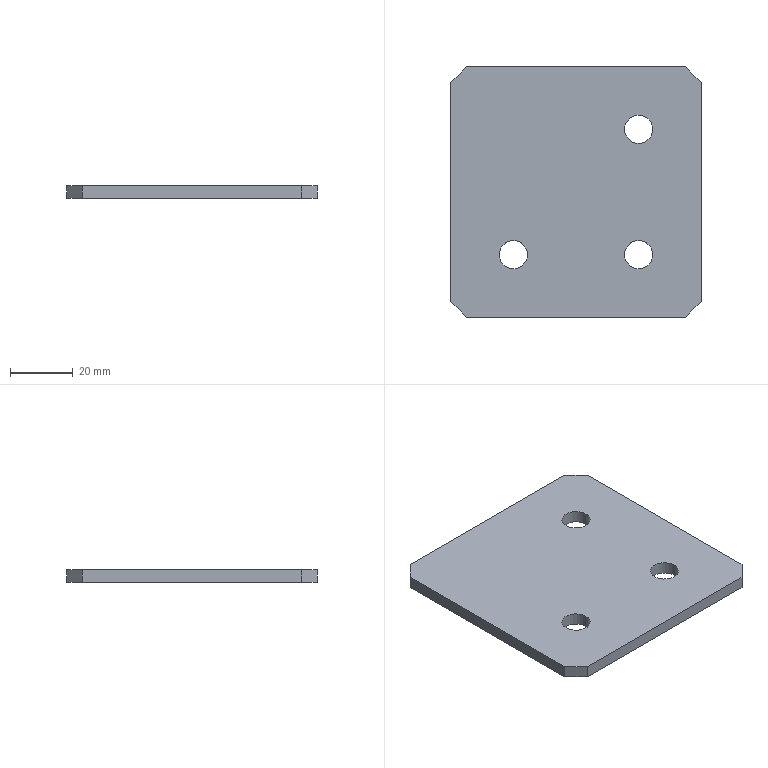Part | SolidWorks | features BaseBody 1 | 1 solid | 16 faces | box 80 x 80 x 4 mm | volume 24637 mm3 | plane 10 | cylinder 6 | commonest cylinder face diameters 9 x6
STEP:
#1=CARTESIAN_POINT('',(55.5,-20.,0.));
#2=VERTEX_POINT('',#1);
#3=CARTESIAN_POINT('',(64.5,-20.,0.));
#4=VERTEX_POINT('',#3);
#5=CARTESIAN_POINT('',(60.,-20.,0.));
#6=DIRECTION('',(0.,0.,1.));
#7=DIRECTION('',(1.,0.,0.));
#8=AXIS2_PLACEMENT_3D('',#5,#6,#7);
#9=CIRCLE('',#8,4.5);
#10=EDGE_CURVE('',#2,#4,#9,.T.);
#11=ORIENTED_EDGE('',*,*,#10,.F.);
#12=CARTESIAN_POINT('',(55.5,-20.,4.));
#13=VERTEX_POINT('',#12);
#14=CARTESIAN_POINT('',(55.5,-20.,4.));
#15=DIRECTION('',(0.,0.,1.));
#16=VECTOR('',#15,1000.);
#17=LINE('',#14,#16);
#18=EDGE_CURVE('',#2,#13,#17,.T.);
#19=ORIENTED_EDGE('',*,*,#18,.T.);
#20=CARTESIAN_POINT('',(64.5,-20.,4.));
#21=VERTEX_POINT('',#20);
#22=CARTESIAN_POINT('',(60.,-20.,4.));
#23=DIRECTION('',(0.,0.,-1.));
#24=DIRECTION('',(1.,0.,0.));
#25=AXIS2_PLACEMENT_3D('',#22,#23,#24);
#26=CIRCLE('',#25,4.5);
#27=EDGE_CURVE('',#21,#13,#26,.T.);
#28=ORIENTED_EDGE('',*,*,#27,.F.);
#29=CARTESIAN_POINT('',(64.5,-20.,4.));
#30=DIRECTION('',(0.,0.,1.));
#31=VECTOR('',#30,1000.);
#32=LINE('',#29,#31);
#33=EDGE_CURVE('',#4,#21,#32,.T.);
#34=ORIENTED_EDGE('',*,*,#33,.F.);
#35=EDGE_LOOP('',(#11,#19,#28,#34));
#36=FACE_OUTER_BOUND('',#35,.T.);
#37=CARTESIAN_POINT('',(60.,-20.,4.));
#38=DIRECTION('',(0.,0.,1.));
#39=DIRECTION('',(1.,0.,0.));
#40=AXIS2_PLACEMENT_3D('',#37,#38,#39);
#41=CYLINDRICAL_SURFACE('',#40,4.5);
#42=ADVANCED_FACE('',(#36),#41,.F.);
#43=CARTESIAN_POINT('',(15.5,-60.,0.));
#44=VERTEX_POINT('',#43);
#45=CARTESIAN_POINT('',(24.5,-60.,0.));
#46=VERTEX_POINT('',#45);
#47=CARTESIAN_POINT('',(20.,-60.,0.));
#48=DIRECTION('',(0.,0.,1.));
#49=DIRECTION('',(1.,0.,0.));
#50=AXIS2_PLACEMENT_3D('',#47,#48,#49);
#51=CIRCLE('',#50,4.5);
#52=EDGE_CURVE('',#44,#46,#51,.T.);
#53=ORIENTED_EDGE('',*,*,#52,.F.);
#54=CARTESIAN_POINT('',(15.5,-60.,4.));
#55=VERTEX_POINT('',#54);
#56=CARTESIAN_POINT('',(15.5,-60.,4.));
#57=DIRECTION('',(0.,0.,1.));
#58=VECTOR('',#57,1000.);
#59=LINE('',#56,#58);
#60=EDGE_CURVE('',#44,#55,#59,.T.);
#61=ORIENTED_EDGE('',*,*,#60,.T.);
#62=CARTESIAN_POINT('',(24.5,-60.,4.));
#63=VERTEX_POINT('',#62);
#64=CARTESIAN_POINT('',(20.,-60.,4.));
#65=DIRECTION('',(0.,0.,-1.));
#66=DIRECTION('',(1.,0.,0.));
#67=AXIS2_PLACEMENT_3D('',#64,#65,#66);
#68=CIRCLE('',#67,4.5);
#69=EDGE_CURVE('',#63,#55,#68,.T.);
#70=ORIENTED_EDGE('',*,*,#69,.F.);
#71=CARTESIAN_POINT('',(24.5,-60.,4.));
#72=DIRECTION('',(0.,0.,1.));
#73=VECTOR('',#72,1000.);
#74=LINE('',#71,#73);
#75=EDGE_CURVE('',#46,#63,#74,.T.);
#76=ORIENTED_EDGE('',*,*,#75,.F.);
#77=EDGE_LOOP('',(#53,#61,#70,#76));
#78=FACE_OUTER_BOUND('',#77,.T.);
#79=CARTESIAN_POINT('',(20.,-60.,4.));
#80=DIRECTION('',(0.,0.,1.));
#81=DIRECTION('',(1.,0.,0.));
#82=AXIS2_PLACEMENT_3D('',#79,#80,#81);
#83=CYLINDRICAL_SURFACE('',#82,4.5);
#84=ADVANCED_FACE('',(#78),#83,.F.);
#85=CARTESIAN_POINT('',(55.5,-60.,0.));
#86=VERTEX_POINT('',#85);
#87=CARTESIAN_POINT('',(64.5,-60.,0.));
#88=VERTEX_POINT('',#87);
#89=CARTESIAN_POINT('',(60.,-60.,0.));
#90=DIRECTION('',(0.,0.,1.));
#91=DIRECTION('',(1.,0.,0.));
#92=AXIS2_PLACEMENT_3D('',#89,#90,#91);
#93=CIRCLE('',#92,4.5);
#94=EDGE_CURVE('',#86,#88,#93,.T.);
#95=ORIENTED_EDGE('',*,*,#94,.F.);
#96=CARTESIAN_POINT('',(55.5,-60.,4.));
#97=VERTEX_POINT('',#96);
#98=CARTESIAN_POINT('',(55.5,-60.,4.));
#99=DIRECTION('',(0.,0.,1.));
#100=VECTOR('',#99,1000.);
#101=LINE('',#98,#100);
#102=EDGE_CURVE('',#86,#97,#101,.T.);
#103=ORIENTED_EDGE('',*,*,#102,.T.);
#104=CARTESIAN_POINT('',(64.5,-60.,4.));
#105=VERTEX_POINT('',#104);
#106=CARTESIAN_POINT('',(60.,-60.,4.));
#107=DIRECTION('',(0.,0.,-1.));
#108=DIRECTION('',(1.,0.,0.));
#109=AXIS2_PLACEMENT_3D('',#106,#107,#108);
#110=CIRCLE('',#109,4.5);
#111=EDGE_CURVE('',#105,#97,#110,.T.);
#112=ORIENTED_EDGE('',*,*,#111,.F.);
#113=CARTESIAN_POINT('',(64.5,-60.,4.));
#114=DIRECTION('',(0.,0.,1.));
#115=VECTOR('',#114,1000.);
#116=LINE('',#113,#115);
#117=EDGE_CURVE('',#88,#105,#116,.T.);
#118=ORIENTED_EDGE('',*,*,#117,.F.);
#119=EDGE_LOOP('',(#95,#103,#112,#118));
#120=FACE_OUTER_BOUND('',#119,.T.);
#121=CARTESIAN_POINT('',(60.,-60.,4.));
#122=DIRECTION('',(0.,0.,1.));
#123=DIRECTION('',(1.,0.,0.));
#124=AXIS2_PLACEMENT_3D('',#121,#122,#123);
#125=CYLINDRICAL_SURFACE('',#124,4.5);
#126=ADVANCED_FACE('',(#120),#125,.F.);
#127=CARTESIAN_POINT('',(0.,-5.,4.));
#128=VERTEX_POINT('',#127);
#129=CARTESIAN_POINT('',(0.,-75.,4.));
#130=VERTEX_POINT('',#129);
#131=CARTESIAN_POINT('',(0.,0.,4.));
#132=DIRECTION('',(0.,-1.,0.));
#133=VECTOR('',#132,1000.);
#134=LINE('',#131,#133);
#135=EDGE_CURVE('',#128,#130,#134,.T.);
#136=ORIENTED_EDGE('',*,*,#135,.T.);
#137=CARTESIAN_POINT('',(5.,-80.,4.));
#138=VERTEX_POINT('',#137);
#139=CARTESIAN_POINT('',(0.,-75.,4.));
#140=DIRECTION('',(0.7071,-0.7071,0.));
#141=VECTOR('',#140,1000.);
#142=LINE('',#139,#141);
#143=EDGE_CURVE('',#130,#138,#142,.T.);
#144=ORIENTED_EDGE('',*,*,#143,.T.);
#145=CARTESIAN_POINT('',(75.,-80.,4.));
#146=VERTEX_POINT('',#145);
#147=CARTESIAN_POINT('',(0.,-80.,4.));
#148=DIRECTION('',(1.,0.,0.));
#149=VECTOR('',#148,1000.);
#150=LINE('',#147,#149);
#151=EDGE_CURVE('',#138,#146,#150,.T.);
#152=ORIENTED_EDGE('',*,*,#151,.T.);
#153=CARTESIAN_POINT('',(80.,-75.,4.));
#154=VERTEX_POINT('',#153);
#155=CARTESIAN_POINT('',(75.,-80.,4.));
#156=DIRECTION('',(0.7071,0.7071,0.));
#157=VECTOR('',#156,1000.);
#158=LINE('',#155,#157);
#159=EDGE_CURVE('',#146,#154,#158,.T.);
#160=ORIENTED_EDGE('',*,*,#159,.T.);
#161=CARTESIAN_POINT('',(80.,-5.,4.));
#162=VERTEX_POINT('',#161);
#163=CARTESIAN_POINT('',(80.,0.,4.));
#164=DIRECTION('',(0.,1.,0.));
#165=VECTOR('',#164,1000.);
#166=LINE('',#163,#165);
#167=EDGE_CURVE('',#154,#162,#166,.T.);
#168=ORIENTED_EDGE('',*,*,#167,.T.);
#169=CARTESIAN_POINT('',(75.,0.,4.));
#170=VERTEX_POINT('',#169);
#171=CARTESIAN_POINT('',(80.,-5.,4.));
#172=DIRECTION('',(-0.7071,0.7071,0.));
#173=VECTOR('',#172,1000.);
#174=LINE('',#171,#173);
#175=EDGE_CURVE('',#162,#170,#174,.T.);
#176=ORIENTED_EDGE('',*,*,#175,.T.);
#177=CARTESIAN_POINT('',(5.,0.,4.));
#178=VERTEX_POINT('',#177);
#179=CARTESIAN_POINT('',(0.,0.,4.));
#180=DIRECTION('',(-1.,0.,0.));
#181=VECTOR('',#180,1000.);
#182=LINE('',#179,#181);
#183=EDGE_CURVE('',#170,#178,#182,.T.);
#184=ORIENTED_EDGE('',*,*,#183,.T.);
#185=CARTESIAN_POINT('',(5.,0.,4.));
#186=DIRECTION('',(-0.7071,-0.7071,0.));
#187=VECTOR('',#186,1000.);
#188=LINE('',#185,#187);
#189=EDGE_CURVE('',#178,#128,#188,.T.);
#190=ORIENTED_EDGE('',*,*,#189,.T.);
#191=EDGE_LOOP('',(#136,#144,#152,#160,#168,#176,#184,#190));
#192=FACE_OUTER_BOUND('',#191,.T.);
#193=ORIENTED_EDGE('',*,*,#27,.T.);
#194=CARTESIAN_POINT('',(60.,-20.,4.));
#195=DIRECTION('',(0.,0.,-1.));
#196=DIRECTION('',(1.,0.,0.));
#197=AXIS2_PLACEMENT_3D('',#194,#195,#196);
#198=CIRCLE('',#197,4.5);
#199=EDGE_CURVE('',#13,#21,#198,.T.);
#200=ORIENTED_EDGE('',*,*,#199,.T.);
#201=EDGE_LOOP('',(#193,#200));
#202=FACE_BOUND('',#201,.T.);
#203=ORIENTED_EDGE('',*,*,#69,.T.);
#204=CARTESIAN_POINT('',(20.,-60.,4.));
#205=DIRECTION('',(0.,0.,-1.));
#206=DIRECTION('',(1.,0.,0.));
#207=AXIS2_PLACEMENT_3D('',#204,#205,#206);
#208=CIRCLE('',#207,4.5);
#209=EDGE_CURVE('',#55,#63,#208,.T.);
#210=ORIENTED_EDGE('',*,*,#209,.T.);
#211=EDGE_LOOP('',(#203,#210));
#212=FACE_BOUND('',#211,.T.);
#213=ORIENTED_EDGE('',*,*,#111,.T.);
#214=CARTESIAN_POINT('',(60.,-60.,4.));
#215=DIRECTION('',(0.,0.,-1.));
#216=DIRECTION('',(1.,0.,0.));
#217=AXIS2_PLACEMENT_3D('',#214,#215,#216);
#218=CIRCLE('',#217,4.5);
#219=EDGE_CURVE('',#97,#105,#218,.T.);
#220=ORIENTED_EDGE('',*,*,#219,.T.);
#221=EDGE_LOOP('',(#213,#220));
#222=FACE_BOUND('',#221,.T.);
#223=CARTESIAN_POINT('',(0.,0.,4.));
#224=DIRECTION('',(0.,0.,1.));
#225=DIRECTION('',(1.,0.,0.));
#226=AXIS2_PLACEMENT_3D('',#223,#224,#225);
#227=PLANE('',#226);
#228=ADVANCED_FACE('',(#192,#202,#212,#222),#227,.T.);
#229=CARTESIAN_POINT('',(0.,-75.,0.));
#230=VERTEX_POINT('',#229);
#231=CARTESIAN_POINT('',(0.,-75.,4.));
#232=DIRECTION('',(0.,0.,1.));
#233=VECTOR('',#232,1000.);
#234=LINE('',#231,#233);
#235=EDGE_CURVE('',#230,#130,#234,.T.);
#236=ORIENTED_EDGE('',*,*,#235,.F.);
#237=CARTESIAN_POINT('',(5.,-80.,0.));
#238=VERTEX_POINT('',#237);
#239=CARTESIAN_POINT('',(5.,-80.,0.));
#240=DIRECTION('',(-0.7071,0.7071,0.));
#241=VECTOR('',#240,1000.);
#242=LINE('',#239,#241);
#243=EDGE_CURVE('',#238,#230,#242,.T.);
#244=ORIENTED_EDGE('',*,*,#243,.F.);
#245=CARTESIAN_POINT('',(5.,-80.,4.));
#246=DIRECTION('',(0.,0.,-1.));
#247=VECTOR('',#246,1000.);
#248=LINE('',#245,#247);
#249=EDGE_CURVE('',#138,#238,#248,.T.);
#250=ORIENTED_EDGE('',*,*,#249,.F.);
#251=ORIENTED_EDGE('',*,*,#143,.F.);
#252=EDGE_LOOP('',(#236,#244,#250,#251));
#253=FACE_OUTER_BOUND('',#252,.T.);
#254=CARTESIAN_POINT('',(5.,-80.,4.));
#255=DIRECTION('',(0.7071,0.7071,0.));
#256=DIRECTION('',(-0.7071,0.7071,0.));
#257=AXIS2_PLACEMENT_3D('',#254,#255,#256);
#258=PLANE('',#257);
#259=ADVANCED_FACE('',(#253),#258,.F.);
#260=ORIENTED_EDGE('',*,*,#235,.T.);
#261=ORIENTED_EDGE('',*,*,#135,.F.);
#262=CARTESIAN_POINT('',(0.,-5.,0.));
#263=VERTEX_POINT('',#262);
#264=CARTESIAN_POINT('',(0.,-5.,4.));
#265=DIRECTION('',(0.,0.,1.));
#266=VECTOR('',#265,1000.);
#267=LINE('',#264,#266);
#268=EDGE_CURVE('',#263,#128,#267,.T.);
#269=ORIENTED_EDGE('',*,*,#268,.F.);
#270=CARTESIAN_POINT('',(0.,0.,0.));
#271=DIRECTION('',(0.,1.,0.));
#272=VECTOR('',#271,1000.);
#273=LINE('',#270,#272);
#274=EDGE_CURVE('',#230,#263,#273,.T.);
#275=ORIENTED_EDGE('',*,*,#274,.F.);
#276=EDGE_LOOP('',(#260,#261,#269,#275));
#277=FACE_OUTER_BOUND('',#276,.T.);
#278=CARTESIAN_POINT('',(0.,0.,4.));
#279=DIRECTION('',(1.,0.,0.));
#280=DIRECTION('',(0.,1.,0.));
#281=AXIS2_PLACEMENT_3D('',#278,#279,#280);
#282=PLANE('',#281);
#283=ADVANCED_FACE('',(#277),#282,.F.);
#284=CARTESIAN_POINT('',(5.,0.,0.));
#285=VERTEX_POINT('',#284);
#286=CARTESIAN_POINT('',(5.,0.,4.));
#287=DIRECTION('',(0.,0.,1.));
#288=VECTOR('',#287,1000.);
#289=LINE('',#286,#288);
#290=EDGE_CURVE('',#285,#178,#289,.T.);
#291=ORIENTED_EDGE('',*,*,#290,.F.);
#292=CARTESIAN_POINT('',(0.,-5.,0.));
#293=DIRECTION('',(0.7071,0.7071,0.));
#294=VECTOR('',#293,1000.);
#295=LINE('',#292,#294);
#296=EDGE_CURVE('',#263,#285,#295,.T.);
#297=ORIENTED_EDGE('',*,*,#296,.F.);
#298=ORIENTED_EDGE('',*,*,#268,.T.);
#299=ORIENTED_EDGE('',*,*,#189,.F.);
#300=EDGE_LOOP('',(#291,#297,#298,#299));
#301=FACE_OUTER_BOUND('',#300,.T.);
#302=CARTESIAN_POINT('',(0.,-5.,4.));
#303=DIRECTION('',(0.7071,-0.7071,0.));
#304=DIRECTION('',(0.7071,0.7071,0.));
#305=AXIS2_PLACEMENT_3D('',#302,#303,#304);
#306=PLANE('',#305);
#307=ADVANCED_FACE('',(#301),#306,.F.);
#308=CARTESIAN_POINT('',(75.,0.,0.));
#309=VERTEX_POINT('',#308);
#310=CARTESIAN_POINT('',(75.,0.,4.));
#311=DIRECTION('',(0.,0.,1.));
#312=VECTOR('',#311,1000.);
#313=LINE('',#310,#312);
#314=EDGE_CURVE('',#309,#170,#313,.T.);
#315=ORIENTED_EDGE('',*,*,#314,.F.);
#316=CARTESIAN_POINT('',(0.,0.,0.));
#317=DIRECTION('',(1.,0.,0.));
#318=VECTOR('',#317,1000.);
#319=LINE('',#316,#318);
#320=EDGE_CURVE('',#285,#309,#319,.T.);
#321=ORIENTED_EDGE('',*,*,#320,.F.);
#322=ORIENTED_EDGE('',*,*,#290,.T.);
#323=ORIENTED_EDGE('',*,*,#183,.F.);
#324=EDGE_LOOP('',(#315,#321,#322,#323));
#325=FACE_OUTER_BOUND('',#324,.T.);
#326=CARTESIAN_POINT('',(0.,0.,4.));
#327=DIRECTION('',(0.,-1.,0.));
#328=DIRECTION('',(0.,0.,-1.));
#329=AXIS2_PLACEMENT_3D('',#326,#327,#328);
#330=PLANE('',#329);
#331=ADVANCED_FACE('',(#325),#330,.F.);
#332=CARTESIAN_POINT('',(80.,-5.,0.));
#333=VERTEX_POINT('',#332);
#334=CARTESIAN_POINT('',(80.,-5.,4.));
#335=DIRECTION('',(0.,0.,1.));
#336=VECTOR('',#335,1000.);
#337=LINE('',#334,#336);
#338=EDGE_CURVE('',#333,#162,#337,.T.);
#339=ORIENTED_EDGE('',*,*,#338,.F.);
#340=CARTESIAN_POINT('',(75.,0.,0.));
#341=DIRECTION('',(0.7071,-0.7071,0.));
#342=VECTOR('',#341,1000.);
#343=LINE('',#340,#342);
#344=EDGE_CURVE('',#309,#333,#343,.T.);
#345=ORIENTED_EDGE('',*,*,#344,.F.);
#346=ORIENTED_EDGE('',*,*,#314,.T.);
#347=ORIENTED_EDGE('',*,*,#175,.F.);
#348=EDGE_LOOP('',(#339,#345,#346,#347));
#349=FACE_OUTER_BOUND('',#348,.T.);
#350=CARTESIAN_POINT('',(75.,0.,4.));
#351=DIRECTION('',(-0.7071,-0.7071,0.));
#352=DIRECTION('',(0.7071,-0.7071,0.));
#353=AXIS2_PLACEMENT_3D('',#350,#351,#352);
#354=PLANE('',#353);
#355=ADVANCED_FACE('',(#349),#354,.F.);
#356=CARTESIAN_POINT('',(80.,-75.,0.));
#357=VERTEX_POINT('',#356);
#358=CARTESIAN_POINT('',(80.,-75.,4.));
#359=DIRECTION('',(0.,0.,1.));
#360=VECTOR('',#359,1000.);
#361=LINE('',#358,#360);
#362=EDGE_CURVE('',#357,#154,#361,.T.);
#363=ORIENTED_EDGE('',*,*,#362,.F.);
#364=CARTESIAN_POINT('',(80.,0.,0.));
#365=DIRECTION('',(0.,-1.,0.));
#366=VECTOR('',#365,1000.);
#367=LINE('',#364,#366);
#368=EDGE_CURVE('',#333,#357,#367,.T.);
#369=ORIENTED_EDGE('',*,*,#368,.F.);
#370=ORIENTED_EDGE('',*,*,#338,.T.);
#371=ORIENTED_EDGE('',*,*,#167,.F.);
#372=EDGE_LOOP('',(#363,#369,#370,#371));
#373=FACE_OUTER_BOUND('',#372,.T.);
#374=CARTESIAN_POINT('',(80.,0.,4.));
#375=DIRECTION('',(-1.,0.,0.));
#376=DIRECTION('',(0.,-1.,0.));
#377=AXIS2_PLACEMENT_3D('',#374,#375,#376);
#378=PLANE('',#377);
#379=ADVANCED_FACE('',(#373),#378,.F.);
#380=CARTESIAN_POINT('',(75.,-80.,0.));
#381=VERTEX_POINT('',#380);
#382=CARTESIAN_POINT('',(75.,-80.,4.));
#383=DIRECTION('',(0.,0.,1.));
#384=VECTOR('',#383,1000.);
#385=LINE('',#382,#384);
#386=EDGE_CURVE('',#381,#146,#385,.T.);
#387=ORIENTED_EDGE('',*,*,#386,.F.);
#388=CARTESIAN_POINT('',(80.,-75.,0.));
#389=DIRECTION('',(-0.7071,-0.7071,0.));
#390=VECTOR('',#389,1000.);
#391=LINE('',#388,#390);
#392=EDGE_CURVE('',#357,#381,#391,.T.);
#393=ORIENTED_EDGE('',*,*,#392,.F.);
#394=ORIENTED_EDGE('',*,*,#362,.T.);
#395=ORIENTED_EDGE('',*,*,#159,.F.);
#396=EDGE_LOOP('',(#387,#393,#394,#395));
#397=FACE_OUTER_BOUND('',#396,.T.);
#398=CARTESIAN_POINT('',(80.,-75.,4.));
#399=DIRECTION('',(-0.7071,0.7071,0.));
#400=DIRECTION('',(-0.7071,-0.7071,0.));
#401=AXIS2_PLACEMENT_3D('',#398,#399,#400);
#402=PLANE('',#401);
#403=ADVANCED_FACE('',(#397),#402,.F.);
#404=ORIENTED_EDGE('',*,*,#386,.T.);
#405=ORIENTED_EDGE('',*,*,#151,.F.);
#406=ORIENTED_EDGE('',*,*,#249,.T.);
#407=CARTESIAN_POINT('',(0.,-80.,0.));
#408=DIRECTION('',(-1.,0.,0.));
#409=VECTOR('',#408,1000.);
#410=LINE('',#407,#409);
#411=EDGE_CURVE('',#381,#238,#410,.T.);
#412=ORIENTED_EDGE('',*,*,#411,.F.);
#413=EDGE_LOOP('',(#404,#405,#406,#412));
#414=FACE_OUTER_BOUND('',#413,.T.);
#415=CARTESIAN_POINT('',(0.,-80.,4.));
#416=DIRECTION('',(0.,1.,0.));
#417=DIRECTION('',(0.,0.,1.));
#418=AXIS2_PLACEMENT_3D('',#415,#416,#417);
#419=PLANE('',#418);
#420=ADVANCED_FACE('',(#414),#419,.F.);
#421=ORIENTED_EDGE('',*,*,#18,.F.);
#422=CARTESIAN_POINT('',(60.,-20.,0.));
#423=DIRECTION('',(0.,0.,1.));
#424=DIRECTION('',(1.,0.,0.));
#425=AXIS2_PLACEMENT_3D('',#422,#423,#424);
#426=CIRCLE('',#425,4.5);
#427=EDGE_CURVE('',#4,#2,#426,.T.);
#428=ORIENTED_EDGE('',*,*,#427,.F.);
#429=ORIENTED_EDGE('',*,*,#33,.T.);
#430=ORIENTED_EDGE('',*,*,#199,.F.);
#431=EDGE_LOOP('',(#421,#428,#429,#430));
#432=FACE_OUTER_BOUND('',#431,.T.);
#433=CARTESIAN_POINT('',(60.,-20.,4.));
#434=DIRECTION('',(0.,0.,1.));
#435=DIRECTION('',(1.,0.,0.));
#436=AXIS2_PLACEMENT_3D('',#433,#434,#435);
#437=CYLINDRICAL_SURFACE('',#436,4.5);
#438=ADVANCED_FACE('',(#432),#437,.F.);
#439=ORIENTED_EDGE('',*,*,#60,.F.);
#440=CARTESIAN_POINT('',(20.,-60.,0.));
#441=DIRECTION('',(0.,0.,1.));
#442=DIRECTION('',(1.,0.,0.));
#443=AXIS2_PLACEMENT_3D('',#440,#441,#442);
#444=CIRCLE('',#443,4.5);
#445=EDGE_CURVE('',#46,#44,#444,.T.);
#446=ORIENTED_EDGE('',*,*,#445,.F.);
#447=ORIENTED_EDGE('',*,*,#75,.T.);
#448=ORIENTED_EDGE('',*,*,#209,.F.);
#449=EDGE_LOOP('',(#439,#446,#447,#448));
#450=FACE_OUTER_BOUND('',#449,.T.);
#451=CARTESIAN_POINT('',(20.,-60.,4.));
#452=DIRECTION('',(0.,0.,1.));
#453=DIRECTION('',(1.,0.,0.));
#454=AXIS2_PLACEMENT_3D('',#451,#452,#453);
#455=CYLINDRICAL_SURFACE('',#454,4.5);
#456=ADVANCED_FACE('',(#450),#455,.F.);
#457=ORIENTED_EDGE('',*,*,#102,.F.);
#458=CARTESIAN_POINT('',(60.,-60.,0.));
#459=DIRECTION('',(0.,0.,1.));
#460=DIRECTION('',(1.,0.,0.));
#461=AXIS2_PLACEMENT_3D('',#458,#459,#460);
#462=CIRCLE('',#461,4.5);
#463=EDGE_CURVE('',#88,#86,#462,.T.);
#464=ORIENTED_EDGE('',*,*,#463,.F.);
#465=ORIENTED_EDGE('',*,*,#117,.T.);
#466=ORIENTED_EDGE('',*,*,#219,.F.);
#467=EDGE_LOOP('',(#457,#464,#465,#466));
#468=FACE_OUTER_BOUND('',#467,.T.);
#469=CARTESIAN_POINT('',(60.,-60.,4.));
#470=DIRECTION('',(0.,0.,1.));
#471=DIRECTION('',(1.,0.,0.));
#472=AXIS2_PLACEMENT_3D('',#469,#470,#471);
#473=CYLINDRICAL_SURFACE('',#472,4.5);
#474=ADVANCED_FACE('',(#468),#473,.F.);
#475=ORIENTED_EDGE('',*,*,#392,.T.);
#476=ORIENTED_EDGE('',*,*,#411,.T.);
#477=ORIENTED_EDGE('',*,*,#243,.T.);
#478=ORIENTED_EDGE('',*,*,#274,.T.);
#479=ORIENTED_EDGE('',*,*,#296,.T.);
#480=ORIENTED_EDGE('',*,*,#320,.T.);
#481=ORIENTED_EDGE('',*,*,#344,.T.);
#482=ORIENTED_EDGE('',*,*,#368,.T.);
#483=EDGE_LOOP('',(#475,#476,#477,#478,#479,#480,#481,#482));
#484=FACE_OUTER_BOUND('',#483,.T.);
#485=ORIENTED_EDGE('',*,*,#427,.T.);
#486=ORIENTED_EDGE('',*,*,#10,.T.);
#487=EDGE_LOOP('',(#485,#486));
#488=FACE_BOUND('',#487,.T.);
#489=ORIENTED_EDGE('',*,*,#445,.T.);
#490=ORIENTED_EDGE('',*,*,#52,.T.);
#491=EDGE_LOOP('',(#489,#490));
#492=FACE_BOUND('',#491,.T.);
#493=ORIENTED_EDGE('',*,*,#463,.T.);
#494=ORIENTED_EDGE('',*,*,#94,.T.);
#495=EDGE_LOOP('',(#493,#494));
#496=FACE_BOUND('',#495,.T.);
#497=CARTESIAN_POINT('',(0.,0.,0.));
#498=DIRECTION('',(0.,0.,1.));
#499=DIRECTION('',(1.,0.,0.));
#500=AXIS2_PLACEMENT_3D('',#497,#498,#499);
#501=PLANE('',#500);
#502=ADVANCED_FACE('',(#484,#488,#492,#496),#501,.F.);
#503=CLOSED_SHELL('',(#42,#84,#126,#228,#259,#283,#307,#331,#355,#379,#403,#420,#438,#456,#474,#502));
#504=MANIFOLD_SOLID_BREP('',#503);
#505=CARTESIAN_POINT('',(0.,0.,0.));
#506=DIRECTION('',(0.,0.,1.));
#507=DIRECTION('',(1.,0.,0.));
#508=AXIS2_PLACEMENT_3D('',#505,#506,#507);
#509=(LENGTH_UNIT()NAMED_UNIT(*)SI_UNIT(.MILLI.,.METRE.));
#510=UNCERTAINTY_MEASURE_WITH_UNIT(LENGTH_MEASURE(0.00001),#509,'','');
#511=(NAMED_UNIT(*)PLANE_ANGLE_UNIT()SI_UNIT($,.RADIAN.));
#512=(NAMED_UNIT(*)SI_UNIT($,.STERADIAN.)SOLID_ANGLE_UNIT());
#513=(GEOMETRIC_REPRESENTATION_CONTEXT(3)GLOBAL_UNCERTAINTY_ASSIGNED_CONTEXT((#510))GLOBAL_UNIT_ASSIGNED_CONTEXT((#509,#511,#512))REPRESENTATION_CONTEXT('',''));
#514=ADVANCED_BREP_SHAPE_REPRESENTATION('',(#504,#508),#513);